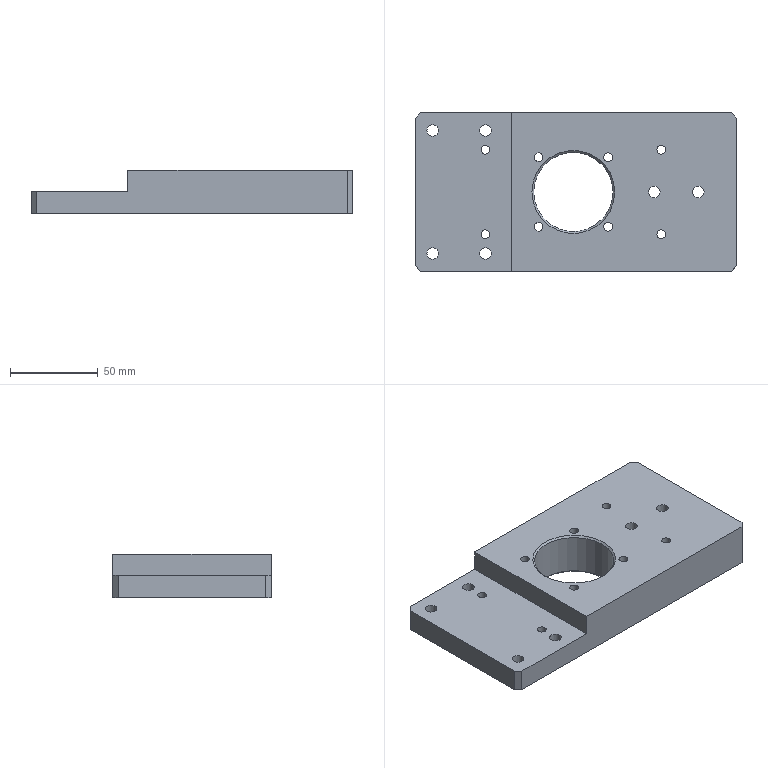CAM job | NX | 3-axis milling, drilling | part box 183 x 90 x 25 mm | stock box 188 x 100 x 30 mm
Tools:
number,name,description,diameter,corner_radius,flute_length,length,flutes
6,D6,平底铣刀-粗,6.0,0.0,25.0,75.0,2
9,D10,平底铣刀-粗,10.0,0.0,35.0,75.0,2
7,D6-J,平底铣刀-精,6.0,0.0,25.0,75.0,2
10,D10-J,平底铣刀-精,10.0,0.0,35.0,75.0,2
1,D80R0.8飞刀,圆鼻刀-粗,80.0,0.8,50.0,75.0,2
1,D80R0.8飞刀-J,圆鼻刀-精,80.0,0.8,50.0,75.0,2
2,D6倒角刀,倒角刀,6.0,0.0,3.0,25.0,2
19,M6X1.0,丝锥,5.0,0.0,35.0,50.0,2
15,ZT5,钻头,5.0,0.0,35.0,50.0,2
17,ZT6.6,钻头,6.6,0.0,35.0,50.0,2
Operations:
program,operation,operation_type,tool,method,geometry_group,spindle_rpm,surface_speed,feed_per_tooth,feed_cut,feed_plunge,cut_length_mm,path_length_mm,cut_time_min,machine_time_min
B,底壁铣飞面开粗_COPY,VolumeBased25DMillingOperation,D80R0.8飞刀,分层开粗-切深K-步距G,W-B,2800.0,703.696,0.5357,3000.0,100.0,5244.277,5554.861,1.748,1.779
B,底壁铣飞面精光_COPY,VolumeBased25DMillingOperation,D80R0.8飞刀-J,侧刃精光-切深K-步距G,W-B,4000.0,1005.28,0.125,1000.0,100.0,582.11,618.11,0.5821,0.5857
B,底壁铣分层开粗-中_COPY,VolumeBased25DMillingOperation,D10,分层开粗-切深K-步距G,W-B,8000.0,251.327,0.3125,5000.0,100.0,17027.329,18064.418,3.405,3.509
B,C0.3封闭铣廓倒角6X45L_COPY,PlanarMilling,D6倒角刀,爬面_倒角-切深0-步距G,W-B,7000.0,131.0,0.1071,1500.0,100.0,150.521,186.521,0.1003,0.1039
B,铣倒角_4,PlanarMilling,D6倒角刀,METHOD,W-B,8000.0,150.796,0.0375,600.0,100.0,113.732,546.701,0.1896,0.2328
B,铣倒角_4_COPY,PlanarMilling,D6倒角刀,METHOD,W-B,8000.0,150.796,0.0375,600.0,100.0,21.936,203.956,0.0366,0.0548
B,平面去毛刺6X45L_COPY,SurfaceContour,D6倒角刀,爬面_倒角-切深0-步距G,W-B,6500.0,122.519,0.1154,1500.0,100.0,874.854,1818.837,0.5832,0.6776
B,底壁铣倒角_COPY,VolumeBased25DMillingOperation,D6倒角刀,爬面_倒角-切深0-步距G,W-B,6500.0,122.519,0.1154,1500.0,100.0,144.527,184.927,0.0964,0.1004
B,底壁铣精光底面-中_COPY,VolumeBased25DMillingOperation,D10-J,精光步距切深关,W-B,8000.0,251.32,0.0625,1000.0,100.0,1247.178,1297.178,1.247,1.252
B,底壁铣精光侧面-中-选底面_COPY,VolumeBased25DMillingOperation,D10-J,侧刃精光-切深K-步距G,W-B,8000.0,251.32,0.0625,1000.0,100.0,108.682,159.682,0.1087,0.1138
A,顶面,FaceMilling,D80R0.8飞刀,侧刃精光-切深K-步距G,W-A,4000.0,1005.31,0.125,1000.0,100.0,888.0,924.0,0.888,0.8916
A,外形粗_2,VolumeBased25DMillingOperation,D10,METHOD,W-A,8000.0,251.327,0.3125,5000.0,80.0,19416.021,19480.021,3.883,3.89
A,底壁铣螺旋开粗-中_COPY,VolumeBased25DMillingOperation,D10,分层开粗-切深K-步距G,W-A,8000.0,251.327,0.1875,3000.0,100.0,4735.162,4797.962,1.578,1.585
A,打点0.8,Operation,D6倒角刀,METHOD,W-A,8000.0,150.796,0.0312,500.0,0.0,1.8,43.6,0.0036,0.0078
A,打点-深0.8,Operation,D6倒角刀,NONE,W-A,8000.0,150.796,0.0312,500.0,90.0,25.2,468.056,0.0504,0.0947
A,通孔-M6螺纹底孔,Operation,ZT5,NONE,W-A,2800.0,43.982,0.0625,350.0,90.0,244.017,784.299,0.6972,0.7512
A,沉头孔-钻孔0段,Operation,ZT6.6,NONE,W-A,1200.0,24.881,0.0625,150.0,90.0,131.897,566.041,0.8793,0.9227
A,铣孔开粗D6_1,CylinderMilling,D6,NONE,W-A,8000.0,150.796,0.075,1200.0,100.0,485.807,603.407,0.4048,0.4166
A,铣孔开粗D6_2,CylinderMilling,D6,NONE,W-A,8000.0,150.796,0.075,1200.0,100.0,923.332,1236.932,0.7694,0.8008
A,铣孔精光D6_1,CylinderMilling,D6-J,精光步距切深关,W-A,8000.0,150.796,0.0312,500.0,100.0,91.868,210.468,0.1837,0.1956
A,铣孔精光D6_2,CylinderMilling,D6-J,精光步距切深关,W-A,8000.0,150.796,0.0312,500.0,100.0,178.461,494.061,0.3569,0.3885
A,仅选体,SurfaceContour,D6倒角刀,METHOD,W-A,8000.0,150.796,0.1875,3000.0,100.0,556.272,592.073,0.1854,0.189
A,铣倒角_1,PlanarMilling,D6倒角刀,METHOD,W-A,8000.0,150.796,0.0312,500.0,100.0,159.505,740.685,0.319,0.3771
A,铣倒角_2,PlanarMilling,D6倒角刀,NONE,W-A,8000.0,150.796,0.05,800.0,100.0,260.356,745.065,0.3254,0.3739
A,铣倒角_3,PlanarMilling,D6倒角刀,METHOD,W-A,8000.0,150.796,0.05,800.0,100.0,145.827,188.827,0.1823,0.1866
A,通孔-攻牙M6,Operation,M6X1.0,METHOD,W-A,500.0,7.854,0.001,1.0,90.0,212.0,720.264,212.0,212.051
A,底壁铣精光侧面-中_COPY,VolumeBased25DMillingOperation,D6-J,侧刃精光-切深K-步距G,W-A,6000.0,113.097,0.0833,1000.0,100.0,647.536,716.963,0.6475,0.6545
A,外形半精_2,VolumeBased25DMillingOperation,D10-J,METHOD,W-A,8000.0,251.327,0.0625,1000.0,100.0,1150.689,1307.704,1.151,1.166